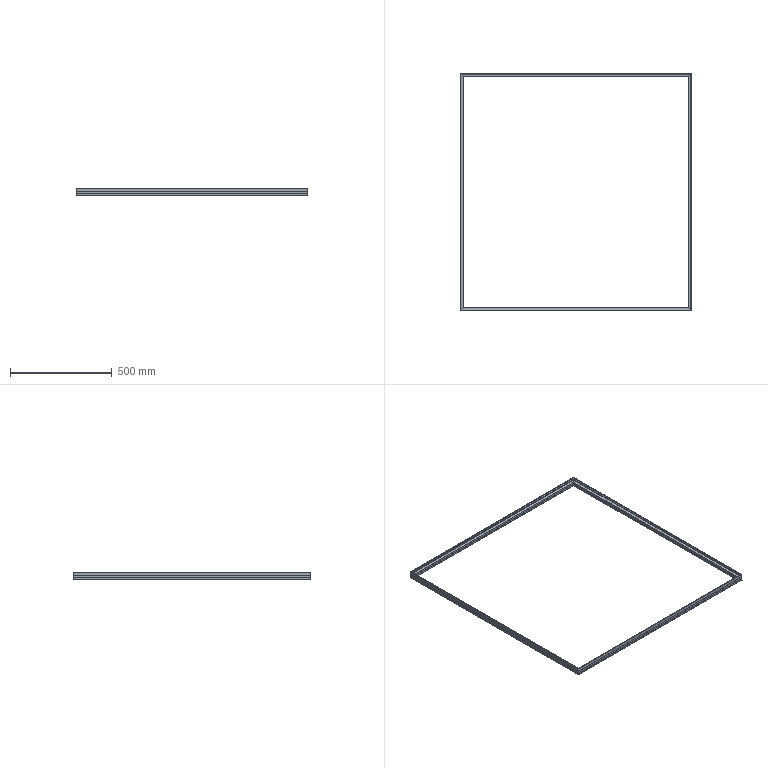Part | 4 solids | 96 faces | box 1140 x 1170 x 35 mm | volume 433005 mm3 | plane 96